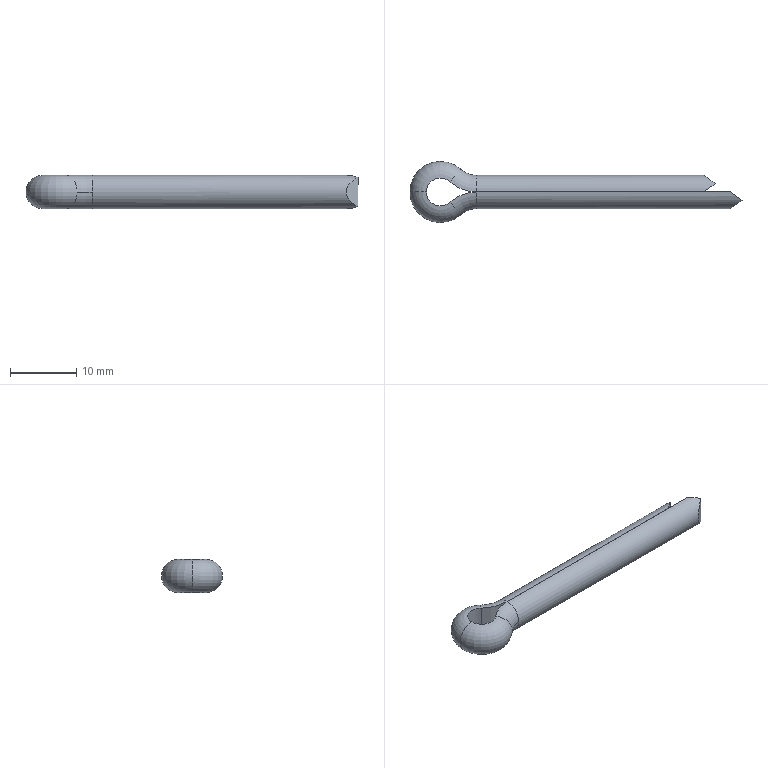Part | SolidWorks | features Cut 1, Sweep 1 | 1 solid | 17 faces | box 50 x 9.2 x 5 mm | volume 942.558 mm3 | torus 6 | plane 6 | cylinder 5 | commonest cylinder face diameters 5 x2 11.782 x2 4.204 x1
STEP:
#1=CARTESIAN_POINT('',(0.,2.5,0.));
#2=VERTEX_POINT('',#1);
#3=CARTESIAN_POINT('',(0.,0.002,2.5));
#4=VERTEX_POINT('',#3);
#5=CARTESIAN_POINT('',(0.,0.,0.));
#6=DIRECTION('',(1.,0.,0.));
#7=DIRECTION('',(0.,0.,-1.));
#8=AXIS2_PLACEMENT_3D('',#5,#6,#7);
#9=CIRCLE('',#8,2.5);
#10=EDGE_CURVE('',#2,#4,#9,.T.);
#11=ORIENTED_EDGE('',*,*,#10,.F.);
#12=CARTESIAN_POINT('',(-2.292,3.391,0.));
#13=VERTEX_POINT('',#12);
#14=CARTESIAN_POINT('',(0.,5.893,0.));
#15=DIRECTION('',(0.,0.,-1.));
#16=DIRECTION('',(-1.,0.,0.));
#17=AXIS2_PLACEMENT_3D('',#14,#15,#16);
#18=CIRCLE('',#17,3.393);
#19=EDGE_CURVE('',#2,#13,#18,.T.);
#20=ORIENTED_EDGE('',*,*,#19,.T.);
#21=CARTESIAN_POINT('',(-3.98,1.55,2.5));
#22=VERTEX_POINT('',#21);
#23=CARTESIAN_POINT('',(-3.981,1.548,0.));
#24=DIRECTION('',(0.7373,-0.6756,0.));
#25=DIRECTION('',(0.,0.,-1.));
#26=AXIS2_PLACEMENT_3D('',#23,#24,#25);
#27=CIRCLE('',#26,2.5);
#28=EDGE_CURVE('',#13,#22,#27,.T.);
#29=ORIENTED_EDGE('',*,*,#28,.T.);
#30=CARTESIAN_POINT('',(0.,5.893,2.5));
#31=DIRECTION('',(0.,0.,-1.));
#32=DIRECTION('',(-1.,0.,0.));
#33=AXIS2_PLACEMENT_3D('',#30,#31,#32);
#34=CIRCLE('',#33,5.891);
#35=EDGE_CURVE('',#4,#22,#34,.T.);
#36=ORIENTED_EDGE('',*,*,#35,.F.);
#37=EDGE_LOOP('',(#11,#20,#29,#36));
#38=FACE_OUTER_BOUND('',#37,.T.);
#39=CARTESIAN_POINT('',(0.,5.893,0.));
#40=DIRECTION('',(0.,0.,-1.));
#41=DIRECTION('',(-1.,0.,0.));
#42=AXIS2_PLACEMENT_3D('',#39,#40,#41);
#43=TOROIDAL_SURFACE('',#42,5.893,2.5);
#44=ADVANCED_FACE('',(#38),#43,.T.);
#45=CARTESIAN_POINT('',(-2.292,-3.391,0.));
#46=VERTEX_POINT('',#45);
#47=CARTESIAN_POINT('',(-3.98,-1.55,2.5));
#48=VERTEX_POINT('',#47);
#49=CARTESIAN_POINT('',(-3.981,-1.548,0.));
#50=DIRECTION('',(-0.7373,-0.6756,0.));
#51=DIRECTION('',(0.,0.,-1.));
#52=AXIS2_PLACEMENT_3D('',#49,#50,#51);
#53=CIRCLE('',#52,2.5);
#54=EDGE_CURVE('',#46,#48,#53,.T.);
#55=ORIENTED_EDGE('',*,*,#54,.F.);
#56=CARTESIAN_POINT('',(0.,-2.5,0.));
#57=VERTEX_POINT('',#56);
#58=CARTESIAN_POINT('',(0.,-5.893,0.));
#59=DIRECTION('',(0.,0.,-1.));
#60=DIRECTION('',(-1.,0.,0.));
#61=AXIS2_PLACEMENT_3D('',#58,#59,#60);
#62=CIRCLE('',#61,3.393);
#63=EDGE_CURVE('',#46,#57,#62,.T.);
#64=ORIENTED_EDGE('',*,*,#63,.T.);
#65=CARTESIAN_POINT('',(0.,-0.002,2.5));
#66=VERTEX_POINT('',#65);
#67=CARTESIAN_POINT('',(0.,0.,0.));
#68=DIRECTION('',(-1.,0.,0.));
#69=DIRECTION('',(0.,0.,-1.));
#70=AXIS2_PLACEMENT_3D('',#67,#68,#69);
#71=CIRCLE('',#70,2.5);
#72=EDGE_CURVE('',#57,#66,#71,.T.);
#73=ORIENTED_EDGE('',*,*,#72,.T.);
#74=CARTESIAN_POINT('',(0.,-5.893,2.5));
#75=DIRECTION('',(0.,0.,-1.));
#76=DIRECTION('',(-1.,0.,0.));
#77=AXIS2_PLACEMENT_3D('',#74,#75,#76);
#78=CIRCLE('',#77,5.891);
#79=EDGE_CURVE('',#48,#66,#78,.T.);
#80=ORIENTED_EDGE('',*,*,#79,.F.);
#81=EDGE_LOOP('',(#55,#64,#73,#80));
#82=FACE_OUTER_BOUND('',#81,.T.);
#83=CARTESIAN_POINT('',(0.,-5.893,0.));
#84=DIRECTION('',(0.,0.,-1.));
#85=DIRECTION('',(-1.,0.,0.));
#86=AXIS2_PLACEMENT_3D('',#83,#84,#85);
#87=TOROIDAL_SURFACE('',#86,5.893,2.5);
#88=ADVANCED_FACE('',(#82),#87,.T.);
#89=CARTESIAN_POINT('',(-3.98,1.55,-2.5));
#90=VERTEX_POINT('',#89);
#91=CARTESIAN_POINT('',(-7.502,0.,-2.5));
#92=VERTEX_POINT('',#91);
#93=CARTESIAN_POINT('',(-5.4,0.,-2.5));
#94=DIRECTION('',(0.,0.,1.));
#95=DIRECTION('',(1.,0.,0.));
#96=AXIS2_PLACEMENT_3D('',#93,#94,#95);
#97=CIRCLE('',#96,2.102);
#98=EDGE_CURVE('',#90,#92,#97,.T.);
#99=ORIENTED_EDGE('',*,*,#98,.T.);
#100=CARTESIAN_POINT('',(-7.502,0.,2.5));
#101=VERTEX_POINT('',#100);
#102=CARTESIAN_POINT('',(-7.5,0.,0.));
#103=DIRECTION('',(0.,1.,0.));
#104=DIRECTION('',(-1.,0.,0.));
#105=AXIS2_PLACEMENT_3D('',#102,#103,#104);
#106=CIRCLE('',#105,2.5);
#107=EDGE_CURVE('',#92,#101,#106,.T.);
#108=ORIENTED_EDGE('',*,*,#107,.T.);
#109=CARTESIAN_POINT('',(-5.4,0.,2.5));
#110=DIRECTION('',(0.,0.,1.));
#111=DIRECTION('',(1.,0.,0.));
#112=AXIS2_PLACEMENT_3D('',#109,#110,#111);
#113=CIRCLE('',#112,2.102);
#114=EDGE_CURVE('',#22,#101,#113,.T.);
#115=ORIENTED_EDGE('',*,*,#114,.F.);
#116=ORIENTED_EDGE('',*,*,#28,.F.);
#117=CARTESIAN_POINT('',(-3.981,1.548,0.));
#118=DIRECTION('',(0.7373,-0.6756,0.));
#119=DIRECTION('',(0.,0.,-1.));
#120=AXIS2_PLACEMENT_3D('',#117,#118,#119);
#121=CIRCLE('',#120,2.5);
#122=EDGE_CURVE('',#90,#13,#121,.T.);
#123=ORIENTED_EDGE('',*,*,#122,.F.);
#124=EDGE_LOOP('',(#99,#108,#115,#116,#123));
#125=FACE_OUTER_BOUND('',#124,.T.);
#126=CARTESIAN_POINT('',(-5.4,0.,0.));
#127=DIRECTION('',(0.,0.,1.));
#128=DIRECTION('',(1.,0.,0.));
#129=AXIS2_PLACEMENT_3D('',#126,#127,#128);
#130=TOROIDAL_SURFACE('',#129,2.1,2.5);
#131=ADVANCED_FACE('',(#125),#130,.T.);
#132=CARTESIAN_POINT('',(38.208,-0.002,2.5));
#133=VERTEX_POINT('',#132);
#134=CARTESIAN_POINT('',(0.,-0.002,2.5));
#135=DIRECTION('',(1.,0.,0.));
#136=VECTOR('',#135,1000.);
#137=LINE('',#134,#136);
#138=EDGE_CURVE('',#66,#133,#137,.T.);
#139=ORIENTED_EDGE('',*,*,#138,.T.);
#140=CARTESIAN_POINT('',(38.208,-0.002,-2.5));
#141=VERTEX_POINT('',#140);
#142=CARTESIAN_POINT('',(38.208,-0.002,2.5));
#143=DIRECTION('',(0.,0.,-1.));
#144=VECTOR('',#143,1000.);
#145=LINE('',#142,#144);
#146=EDGE_CURVE('',#133,#141,#145,.T.);
#147=ORIENTED_EDGE('',*,*,#146,.T.);
#148=CARTESIAN_POINT('',(0.,-0.002,-2.5));
#149=VERTEX_POINT('',#148);
#150=CARTESIAN_POINT('',(0.,-0.002,-2.5));
#151=DIRECTION('',(1.,0.,0.));
#152=VECTOR('',#151,1000.);
#153=LINE('',#150,#152);
#154=EDGE_CURVE('',#149,#141,#153,.T.);
#155=ORIENTED_EDGE('',*,*,#154,.F.);
#156=CARTESIAN_POINT('',(0.,-0.002,2.5));
#157=DIRECTION('',(0.,0.,-1.));
#158=VECTOR('',#157,1000.);
#159=LINE('',#156,#158);
#160=EDGE_CURVE('',#66,#149,#159,.T.);
#161=ORIENTED_EDGE('',*,*,#160,.F.);
#162=EDGE_LOOP('',(#139,#147,#155,#161));
#163=FACE_OUTER_BOUND('',#162,.T.);
#164=CARTESIAN_POINT('',(0.,-0.002,2.5));
#165=DIRECTION('',(0.,-1.,0.));
#166=DIRECTION('',(1.,0.,0.));
#167=AXIS2_PLACEMENT_3D('',#164,#165,#166);
#168=PLANE('',#167);
#169=ADVANCED_FACE('',(#163),#168,.F.);
#170=CARTESIAN_POINT('',(40.,-1.251,-2.164));
#171=VERTEX_POINT('',#170);
#172=CARTESIAN_POINT('',(40.,-1.251,2.164));
#173=VERTEX_POINT('',#172);
#174=CARTESIAN_POINT('',(40.,-1.251,-2.164));
#175=CARTESIAN_POINT('',(37.337,-3.124,-1.082));
#176=CARTESIAN_POINT('',(37.337,-3.124,1.082));
#177=CARTESIAN_POINT('',(40.,-1.251,2.164));
#178=(BOUNDED_CURVE()B_SPLINE_CURVE(3,(#174,#175,#176,#177),.UNSPECIFIED.,.F.,.F.)B_SPLINE_CURVE_WITH_KNOTS((4,4),(2.095,4.188),.UNSPECIFIED.)CURVE()GEOMETRIC_REPRESENTATION_ITEM()RATIONAL_B_SPLINE_CURVE((1.,0.6669,0.6669,1.))REPRESENTATION_ITEM(''));
#179=EDGE_CURVE('',#171,#173,#178,.T.);
#180=ORIENTED_EDGE('',*,*,#179,.T.);
#181=CARTESIAN_POINT('',(40.,-1.251,2.164));
#182=CARTESIAN_POINT('',(39.452,-0.8691,2.385));
#183=CARTESIAN_POINT('',(38.841,-0.4431,2.5));
#184=CARTESIAN_POINT('',(38.208,-0.002,2.5));
#185=(BOUNDED_CURVE()B_SPLINE_CURVE(3,(#181,#182,#183,#184),.UNSPECIFIED.,.F.,.F.)B_SPLINE_CURVE_WITH_KNOTS((4,4),(1.047,1.57),.UNSPECIFIED.)CURVE()GEOMETRIC_REPRESENTATION_ITEM()RATIONAL_B_SPLINE_CURVE((1.,0.9773,0.9773,1.))REPRESENTATION_ITEM(''));
#186=EDGE_CURVE('',#173,#133,#185,.T.);
#187=ORIENTED_EDGE('',*,*,#186,.T.);
#188=ORIENTED_EDGE('',*,*,#138,.F.);
#189=ORIENTED_EDGE('',*,*,#72,.F.);
#190=CARTESIAN_POINT('',(0.,0.,0.));
#191=DIRECTION('',(-1.,0.,0.));
#192=DIRECTION('',(0.,0.,-1.));
#193=AXIS2_PLACEMENT_3D('',#190,#191,#192);
#194=CIRCLE('',#193,2.5);
#195=EDGE_CURVE('',#149,#57,#194,.T.);
#196=ORIENTED_EDGE('',*,*,#195,.F.);
#197=ORIENTED_EDGE('',*,*,#154,.T.);
#198=CARTESIAN_POINT('',(38.208,-0.002,-2.5));
#199=CARTESIAN_POINT('',(38.841,-0.4431,-2.5));
#200=CARTESIAN_POINT('',(39.452,-0.8691,-2.385));
#201=CARTESIAN_POINT('',(40.,-1.251,-2.164));
#202=(BOUNDED_CURVE()B_SPLINE_CURVE(3,(#198,#199,#200,#201),.UNSPECIFIED.,.F.,.F.)B_SPLINE_CURVE_WITH_KNOTS((4,4),(4.713,5.236),.UNSPECIFIED.)CURVE()GEOMETRIC_REPRESENTATION_ITEM()RATIONAL_B_SPLINE_CURVE((1.,0.9773,0.9773,1.))REPRESENTATION_ITEM(''));
#203=EDGE_CURVE('',#141,#171,#202,.T.);
#204=ORIENTED_EDGE('',*,*,#203,.T.);
#205=EDGE_LOOP('',(#180,#187,#188,#189,#196,#197,#204));
#206=FACE_OUTER_BOUND('',#205,.T.);
#207=CARTESIAN_POINT('',(0.,0.,0.));
#208=DIRECTION('',(1.,0.,0.));
#209=DIRECTION('',(0.,1.,0.));
#210=AXIS2_PLACEMENT_3D('',#207,#208,#209);
#211=CYLINDRICAL_SURFACE('',#210,2.5);
#212=ADVANCED_FACE('',(#206),#211,.T.);
#213=CARTESIAN_POINT('',(-3.98,-1.55,-2.5));
#214=VERTEX_POINT('',#213);
#215=CARTESIAN_POINT('',(-3.98,-1.55,2.5));
#216=DIRECTION('',(0.,0.,-1.));
#217=VECTOR('',#216,1000.);
#218=LINE('',#215,#217);
#219=EDGE_CURVE('',#48,#214,#218,.T.);
#220=ORIENTED_EDGE('',*,*,#219,.F.);
#221=ORIENTED_EDGE('',*,*,#79,.T.);
#222=ORIENTED_EDGE('',*,*,#160,.T.);
#223=CARTESIAN_POINT('',(0.,-5.893,-2.5));
#224=DIRECTION('',(0.,0.,-1.));
#225=DIRECTION('',(-1.,0.,0.));
#226=AXIS2_PLACEMENT_3D('',#223,#224,#225);
#227=CIRCLE('',#226,5.891);
#228=EDGE_CURVE('',#214,#149,#227,.T.);
#229=ORIENTED_EDGE('',*,*,#228,.F.);
#230=EDGE_LOOP('',(#220,#221,#222,#229));
#231=FACE_OUTER_BOUND('',#230,.T.);
#232=CARTESIAN_POINT('',(0.,-5.893,0.));
#233=DIRECTION('',(0.,0.,-1.));
#234=DIRECTION('',(-1.,0.,0.));
#235=AXIS2_PLACEMENT_3D('',#232,#233,#234);
#236=CYLINDRICAL_SURFACE('',#235,5.891);
#237=ADVANCED_FACE('',(#231),#236,.T.);
#238=ORIENTED_EDGE('',*,*,#63,.F.);
#239=CARTESIAN_POINT('',(-3.981,-1.548,0.));
#240=DIRECTION('',(-0.7373,-0.6756,0.));
#241=DIRECTION('',(0.,0.,-1.));
#242=AXIS2_PLACEMENT_3D('',#239,#240,#241);
#243=CIRCLE('',#242,2.5);
#244=EDGE_CURVE('',#214,#46,#243,.T.);
#245=ORIENTED_EDGE('',*,*,#244,.F.);
#246=ORIENTED_EDGE('',*,*,#228,.T.);
#247=ORIENTED_EDGE('',*,*,#195,.T.);
#248=EDGE_LOOP('',(#238,#245,#246,#247));
#249=FACE_OUTER_BOUND('',#248,.T.);
#250=CARTESIAN_POINT('',(0.,-5.893,0.));
#251=DIRECTION('',(0.,0.,-1.));
#252=DIRECTION('',(-1.,0.,0.));
#253=AXIS2_PLACEMENT_3D('',#250,#251,#252);
#254=TOROIDAL_SURFACE('',#253,5.893,2.5);
#255=ADVANCED_FACE('',(#249),#254,.T.);
#256=CARTESIAN_POINT('',(-3.98,1.55,2.5));
#257=DIRECTION('',(0.,0.,-1.));
#258=VECTOR('',#257,1000.);
#259=LINE('',#256,#258);
#260=EDGE_CURVE('',#22,#90,#259,.T.);
#261=ORIENTED_EDGE('',*,*,#260,.F.);
#262=ORIENTED_EDGE('',*,*,#114,.T.);
#263=CARTESIAN_POINT('',(-5.4,0.,2.5));
#264=DIRECTION('',(0.,0.,1.));
#265=DIRECTION('',(1.,0.,0.));
#266=AXIS2_PLACEMENT_3D('',#263,#264,#265);
#267=CIRCLE('',#266,2.102);
#268=EDGE_CURVE('',#101,#48,#267,.T.);
#269=ORIENTED_EDGE('',*,*,#268,.T.);
#270=ORIENTED_EDGE('',*,*,#219,.T.);
#271=CARTESIAN_POINT('',(-5.4,0.,-2.5));
#272=DIRECTION('',(0.,0.,1.));
#273=DIRECTION('',(1.,0.,0.));
#274=AXIS2_PLACEMENT_3D('',#271,#272,#273);
#275=CIRCLE('',#274,2.102);
#276=EDGE_CURVE('',#92,#214,#275,.T.);
#277=ORIENTED_EDGE('',*,*,#276,.F.);
#278=ORIENTED_EDGE('',*,*,#98,.F.);
#279=EDGE_LOOP('',(#261,#262,#269,#270,#277,#278));
#280=FACE_OUTER_BOUND('',#279,.T.);
#281=CARTESIAN_POINT('',(-5.4,0.,0.));
#282=DIRECTION('',(0.,0.,1.));
#283=DIRECTION('',(1.,0.,0.));
#284=AXIS2_PLACEMENT_3D('',#281,#282,#283);
#285=CYLINDRICAL_SURFACE('',#284,2.102);
#286=ADVANCED_FACE('',(#280),#285,.F.);
#287=ORIENTED_EDGE('',*,*,#107,.F.);
#288=ORIENTED_EDGE('',*,*,#276,.T.);
#289=ORIENTED_EDGE('',*,*,#244,.T.);
#290=ORIENTED_EDGE('',*,*,#54,.T.);
#291=ORIENTED_EDGE('',*,*,#268,.F.);
#292=EDGE_LOOP('',(#287,#288,#289,#290,#291));
#293=FACE_OUTER_BOUND('',#292,.T.);
#294=CARTESIAN_POINT('',(-5.4,0.,0.));
#295=DIRECTION('',(0.,0.,1.));
#296=DIRECTION('',(1.,0.,0.));
#297=AXIS2_PLACEMENT_3D('',#294,#295,#296);
#298=TOROIDAL_SURFACE('',#297,2.1,2.5);
#299=ADVANCED_FACE('',(#293),#298,.T.);
#300=CARTESIAN_POINT('',(0.,0.002,-2.5));
#301=VERTEX_POINT('',#300);
#302=CARTESIAN_POINT('',(0.,0.002,2.5));
#303=DIRECTION('',(0.,0.,-1.));
#304=VECTOR('',#303,1000.);
#305=LINE('',#302,#304);
#306=EDGE_CURVE('',#4,#301,#305,.T.);
#307=ORIENTED_EDGE('',*,*,#306,.F.);
#308=ORIENTED_EDGE('',*,*,#35,.T.);
#309=ORIENTED_EDGE('',*,*,#260,.T.);
#310=CARTESIAN_POINT('',(0.,5.893,-2.5));
#311=DIRECTION('',(0.,0.,-1.));
#312=DIRECTION('',(-1.,0.,0.));
#313=AXIS2_PLACEMENT_3D('',#310,#311,#312);
#314=CIRCLE('',#313,5.891);
#315=EDGE_CURVE('',#301,#90,#314,.T.);
#316=ORIENTED_EDGE('',*,*,#315,.F.);
#317=EDGE_LOOP('',(#307,#308,#309,#316));
#318=FACE_OUTER_BOUND('',#317,.T.);
#319=CARTESIAN_POINT('',(0.,5.893,0.));
#320=DIRECTION('',(0.,0.,-1.));
#321=DIRECTION('',(-1.,0.,0.));
#322=AXIS2_PLACEMENT_3D('',#319,#320,#321);
#323=CYLINDRICAL_SURFACE('',#322,5.891);
#324=ADVANCED_FACE('',(#318),#323,.T.);
#325=ORIENTED_EDGE('',*,*,#19,.F.);
#326=CARTESIAN_POINT('',(0.,0.,0.));
#327=DIRECTION('',(1.,0.,0.));
#328=DIRECTION('',(0.,0.,-1.));
#329=AXIS2_PLACEMENT_3D('',#326,#327,#328);
#330=CIRCLE('',#329,2.5);
#331=EDGE_CURVE('',#301,#2,#330,.T.);
#332=ORIENTED_EDGE('',*,*,#331,.F.);
#333=ORIENTED_EDGE('',*,*,#315,.T.);
#334=ORIENTED_EDGE('',*,*,#122,.T.);
#335=EDGE_LOOP('',(#325,#332,#333,#334));
#336=FACE_OUTER_BOUND('',#335,.T.);
#337=CARTESIAN_POINT('',(0.,5.893,0.));
#338=DIRECTION('',(0.,0.,-1.));
#339=DIRECTION('',(-1.,0.,0.));
#340=AXIS2_PLACEMENT_3D('',#337,#338,#339);
#341=TOROIDAL_SURFACE('',#340,5.893,2.5);
#342=ADVANCED_FACE('',(#336),#341,.T.);
#343=CARTESIAN_POINT('',(36.,1.251,2.164));
#344=VERTEX_POINT('',#343);
#345=CARTESIAN_POINT('',(34.208,0.002,2.5));
#346=VERTEX_POINT('',#345);
#347=CARTESIAN_POINT('',(36.,1.251,2.164));
#348=CARTESIAN_POINT('',(35.452,0.8691,2.385));
#349=CARTESIAN_POINT('',(34.841,0.4431,2.5));
#350=CARTESIAN_POINT('',(34.208,0.002,2.5));
#351=(BOUNDED_CURVE()B_SPLINE_CURVE(3,(#347,#348,#349,#350),.UNSPECIFIED.,.F.,.F.)B_SPLINE_CURVE_WITH_KNOTS((4,4),(1.047,1.57),.UNSPECIFIED.)CURVE()GEOMETRIC_REPRESENTATION_ITEM()RATIONAL_B_SPLINE_CURVE((1.,0.9773,0.9773,1.))REPRESENTATION_ITEM(''));
#352=EDGE_CURVE('',#344,#346,#351,.T.);
#353=ORIENTED_EDGE('',*,*,#352,.F.);
#354=CARTESIAN_POINT('',(36.,1.251,-2.164));
#355=VERTEX_POINT('',#354);
#356=CARTESIAN_POINT('',(36.,1.251,-2.164));
#357=CARTESIAN_POINT('',(33.337,3.124,-1.082));
#358=CARTESIAN_POINT('',(33.337,3.124,1.082));
#359=CARTESIAN_POINT('',(36.,1.251,2.164));
#360=(BOUNDED_CURVE()B_SPLINE_CURVE(3,(#356,#357,#358,#359),.UNSPECIFIED.,.F.,.F.)B_SPLINE_CURVE_WITH_KNOTS((4,4),(2.095,4.188),.UNSPECIFIED.)CURVE()GEOMETRIC_REPRESENTATION_ITEM()RATIONAL_B_SPLINE_CURVE((1.,0.6669,0.6669,1.))REPRESENTATION_ITEM(''));
#361=EDGE_CURVE('',#355,#344,#360,.T.);
#362=ORIENTED_EDGE('',*,*,#361,.F.);
#363=CARTESIAN_POINT('',(34.208,0.002,-2.5));
#364=VERTEX_POINT('',#363);
#365=CARTESIAN_POINT('',(34.208,0.002,-2.5));
#366=CARTESIAN_POINT('',(34.841,0.4431,-2.5));
#367=CARTESIAN_POINT('',(35.452,0.8691,-2.385));
#368=CARTESIAN_POINT('',(36.,1.251,-2.164));
#369=(BOUNDED_CURVE()B_SPLINE_CURVE(3,(#365,#366,#367,#368),.UNSPECIFIED.,.F.,.T.)B_SPLINE_CURVE_WITH_KNOTS((4,4),(4.713,5.236),.UNSPECIFIED.)CURVE()GEOMETRIC_REPRESENTATION_ITEM()RATIONAL_B_SPLINE_CURVE((1.,0.9773,0.9773,1.))REPRESENTATION_ITEM(''));
#370=EDGE_CURVE('',#364,#355,#369,.T.);
#371=ORIENTED_EDGE('',*,*,#370,.F.);
#372=CARTESIAN_POINT('',(0.,0.002,-2.5));
#373=DIRECTION('',(1.,0.,0.));
#374=VECTOR('',#373,1000.);
#375=LINE('',#372,#374);
#376=EDGE_CURVE('',#301,#364,#375,.T.);
#377=ORIENTED_EDGE('',*,*,#376,.F.);
#378=ORIENTED_EDGE('',*,*,#331,.T.);
#379=ORIENTED_EDGE('',*,*,#10,.T.);
#380=CARTESIAN_POINT('',(0.,0.002,2.5));
#381=DIRECTION('',(1.,0.,0.));
#382=VECTOR('',#381,1000.);
#383=LINE('',#380,#382);
#384=EDGE_CURVE('',#4,#346,#383,.T.);
#385=ORIENTED_EDGE('',*,*,#384,.T.);
#386=EDGE_LOOP('',(#353,#362,#371,#377,#378,#379,#385));
#387=FACE_OUTER_BOUND('',#386,.T.);
#388=CARTESIAN_POINT('',(0.,0.,0.));
#389=DIRECTION('',(1.,0.,0.));
#390=DIRECTION('',(0.,0.,-1.));
#391=AXIS2_PLACEMENT_3D('',#388,#389,#390);
#392=CYLINDRICAL_SURFACE('',#391,2.5);
#393=ADVANCED_FACE('',(#387),#392,.T.);
#394=CARTESIAN_POINT('',(34.208,0.002,2.5));
#395=DIRECTION('',(0.,0.,-1.));
#396=VECTOR('',#395,1000.);
#397=LINE('',#394,#396);
#398=EDGE_CURVE('',#346,#364,#397,.T.);
#399=ORIENTED_EDGE('',*,*,#398,.F.);
#400=ORIENTED_EDGE('',*,*,#384,.F.);
#401=ORIENTED_EDGE('',*,*,#306,.T.);
#402=ORIENTED_EDGE('',*,*,#376,.T.);
#403=EDGE_LOOP('',(#399,#400,#401,#402));
#404=FACE_OUTER_BOUND('',#403,.T.);
#405=CARTESIAN_POINT('',(0.,0.002,2.5));
#406=DIRECTION('',(0.,-1.,0.));
#407=DIRECTION('',(0.,0.,-1.));
#408=AXIS2_PLACEMENT_3D('',#405,#406,#407);
#409=PLANE('',#408);
#410=ADVANCED_FACE('',(#404),#409,.T.);
#411=ORIENTED_EDGE('',*,*,#352,.T.);
#412=ORIENTED_EDGE('',*,*,#398,.T.);
#413=ORIENTED_EDGE('',*,*,#370,.T.);
#414=CARTESIAN_POINT('',(36.,1.251,-2.5));
#415=DIRECTION('',(0.,0.,1.));
#416=VECTOR('',#415,1000.);
#417=LINE('',#414,#416);
#418=EDGE_CURVE('',#355,#344,#417,.T.);
#419=ORIENTED_EDGE('',*,*,#418,.T.);
#420=EDGE_LOOP('',(#411,#412,#413,#419));
#421=FACE_OUTER_BOUND('',#420,.T.);
#422=CARTESIAN_POINT('',(36.,1.251,-2.5));
#423=DIRECTION('',(-0.5717,0.8204,0.));
#424=DIRECTION('',(-0.8204,-0.5717,0.));
#425=AXIS2_PLACEMENT_3D('',#422,#423,#424);
#426=PLANE('',#425);
#427=ADVANCED_FACE('',(#421),#426,.F.);
#428=ORIENTED_EDGE('',*,*,#361,.T.);
#429=ORIENTED_EDGE('',*,*,#418,.F.);
#430=EDGE_LOOP('',(#428,#429));
#431=FACE_OUTER_BOUND('',#430,.T.);
#432=CARTESIAN_POINT('',(36.,1.251,-2.5));
#433=DIRECTION('',(-0.5754,-0.8179,0.));
#434=DIRECTION('',(0.8179,-0.5754,0.));
#435=AXIS2_PLACEMENT_3D('',#432,#433,#434);
#436=PLANE('',#435);
#437=ADVANCED_FACE('',(#431),#436,.F.);
#438=CARTESIAN_POINT('',(40.,-1.251,-2.5));
#439=DIRECTION('',(0.,0.,1.));
#440=VECTOR('',#439,1000.);
#441=LINE('',#438,#440);
#442=EDGE_CURVE('',#171,#173,#441,.T.);
#443=ORIENTED_EDGE('',*,*,#442,.T.);
#444=ORIENTED_EDGE('',*,*,#179,.F.);
#445=EDGE_LOOP('',(#443,#444));
#446=FACE_OUTER_BOUND('',#445,.T.);
#447=CARTESIAN_POINT('',(40.,-1.251,-2.5));
#448=DIRECTION('',(-0.5754,0.8179,0.));
#449=DIRECTION('',(-0.8179,-0.5754,0.));
#450=AXIS2_PLACEMENT_3D('',#447,#448,#449);
#451=PLANE('',#450);
#452=ADVANCED_FACE('',(#446),#451,.F.);
#453=ORIENTED_EDGE('',*,*,#442,.F.);
#454=ORIENTED_EDGE('',*,*,#203,.F.);
#455=ORIENTED_EDGE('',*,*,#146,.F.);
#456=ORIENTED_EDGE('',*,*,#186,.F.);
#457=EDGE_LOOP('',(#453,#454,#455,#456));
#458=FACE_OUTER_BOUND('',#457,.T.);
#459=CARTESIAN_POINT('',(40.,-1.251,-2.5));
#460=DIRECTION('',(-0.5717,-0.8204,0.));
#461=DIRECTION('',(0.8204,-0.5717,0.));
#462=AXIS2_PLACEMENT_3D('',#459,#460,#461);
#463=PLANE('',#462);
#464=ADVANCED_FACE('',(#458),#463,.F.);
#465=CLOSED_SHELL('',(#44,#88,#131,#169,#212,#237,#255,#286,#299,#324,#342,#393,#410,#427,#437,#452,#464));
#466=MANIFOLD_SOLID_BREP('',#465);
#467=CARTESIAN_POINT('',(0.,0.,0.));
#468=DIRECTION('',(0.,0.,1.));
#469=DIRECTION('',(1.,0.,0.));
#470=AXIS2_PLACEMENT_3D('',#467,#468,#469);
#471=(LENGTH_UNIT()NAMED_UNIT(*)SI_UNIT(.MILLI.,.METRE.));
#472=UNCERTAINTY_MEASURE_WITH_UNIT(LENGTH_MEASURE(0.00001),#471,'','');
#473=(NAMED_UNIT(*)PLANE_ANGLE_UNIT()SI_UNIT($,.RADIAN.));
#474=(NAMED_UNIT(*)SI_UNIT($,.STERADIAN.)SOLID_ANGLE_UNIT());
#475=(GEOMETRIC_REPRESENTATION_CONTEXT(3)GLOBAL_UNCERTAINTY_ASSIGNED_CONTEXT((#472))GLOBAL_UNIT_ASSIGNED_CONTEXT((#471,#473,#474))REPRESENTATION_CONTEXT('',''));
#476=ADVANCED_BREP_SHAPE_REPRESENTATION('',(#466,#470),#475);